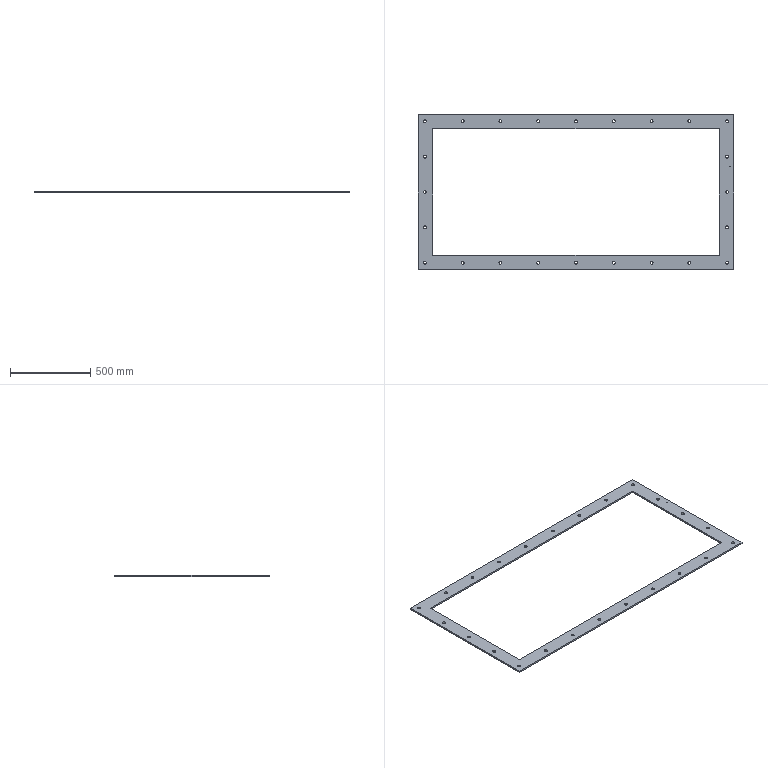Part | STEP file | Feed inlet flange_Default<As machined> | 1 solid | 60 faces | box 1960 x 960 x 10 mm | volume 4768318 mm3 | cylinder 50 | plane 10 | commonest cylinder face diameters 18 x48 2.5 x2